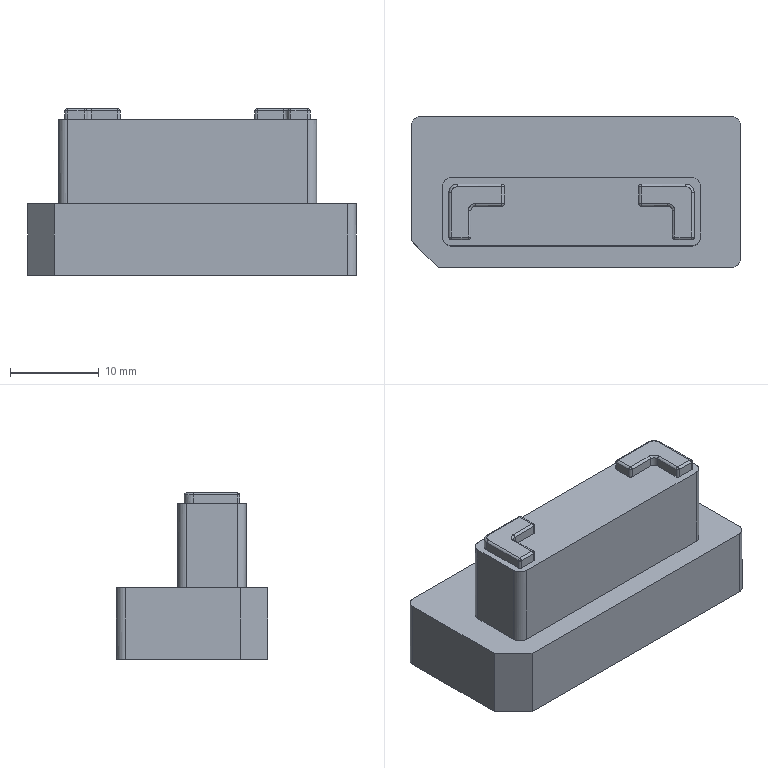NC program | PowerMill | posted with a generic post | part box 37 x 17 x 18.689 mm
Lines 1 to 1026 of 30982:
%
O0001
N104 ( POWERMILL CB  : 2026004.0)
N105 ( POST VER      : 2026.0.0.5161)
N106 ( OPTION FILE   : FANUC)
N107 ( OUTPUT WORKPLANE : WORLD)
N108 (  )
N109 ( TOOL LIST )
N110 (---------------------------------------)
N111 ( NO. | ID        | DIA.| TIP RAD|LENGTH)
N112 (---------------------------------------)
N113 (    1|D10C_1_1_1 |10.0 |  0.0   |74.16 )
N114 (    2|D4C_1      | 4.0 |  0.0   | 59.0 )
N115 (    3|D10_1_1_1  |10.0 |  0.0   |73.84 )
N116 (   10|D3_1       | 3.0 |  0.0   | 58.0 )
N117 (    8|D1_1_1     | 1.0 |  0.0   |56.48 )
N118 (   13|TEXT_D4_1_1| 4.0 |  0.3   |65.96 )
N119 (---------------------------------------)
N120 (  )
N121 ( NUMBER OF TOOLPATHS: 12.0 )
N122 ( ESTIMATED PROGRAM DURATION: 0 HOURS 5 MIN 14 SEC)
N123 (  )
N124 G00 G21 G80 G40 G17
N125 G90
N126 G54
N127 G53 Z0.0
N128 (---------------)
N129 ( START TOOLPATH : 精公开粗01-扫面平行-D10C )
N130 (---------------)
N131 ( TOOL NO.    :1 )
N132 ( TOOL TYPE   : ENDMILL)
N133 ( TOOL ID     : D10C_1_1_1)
N134 ( TOOL DIA    : 10.0 LENGTH 74.16)
N135 T1
N136 M6
N137 S8000 M03
N138 G00 G90 X0.0 Y0.0
N139 G43 Z10.2 H1
N140
N141 G05 P10000 R4
N142 X26.28 Y11.28
N143 Z1.129
N144 G01 Z-0.071 F6000.0
N145 X21.28 F10000.0
N146 X-21.28
N147 Y5.64
N148 X21.28
N149 Y0.0
N150 X-21.28
N151 Y-5.64
N152 X21.28
N153 Y-11.28
N154 X-21.28
N155 X-26.28
N156 G00 Z10.2
N157 G05 P0
N158 (---------------)
N159 ( END TOOLPATH : 精公开粗01-扫面平行-D10C )
N160 (---------------)
N161 ( START TOOLPATH : 精公开粗01-外形偏置-D10C )
N162 (---------------)
N163 G00 X-0.5005 Y-1.2945 Z9.879
N164 G05 P10000 R4
N165 X-28.071 Y-7.1954
N166 Z0.6887
N167 G01 Z-0.5113 F6000.0
N168 X-27.5435 F10000.0
N169 G03 X-22.796 Y-2.4479 I0.0 J4.7475
N170 G01 Y10.28
N171 G02 X-21.796 Y11.28 I1.0 J0.0
N172 G01 X20.795
N173 G02 X21.795 Y10.28 I0.0 J-1.0
N174 G01 Y-2.4477
N175 X18.5751 Y-2.4546
N176 X18.581 Y-5.1616
N177 X18.5136 Y-5.9351
N178 X18.3397 Y-6.7085
N179 X18.0411 Y-7.4819
N180 X17.675 Y-8.1342
N181 X16.9485 Y-9.0288
N182 X16.1282 Y-9.7035
N183 X15.3547 Y-10.1401
N184 X14.5813 Y-10.4291
N185 X13.9308 Y-10.5756
N186 X13.0345 Y-10.6552
N187 X10.7142 Y-10.6411
N188 X9.9408 Y-10.5315
N189 X9.1673 Y-10.3059
N190 X8.3939 Y-9.9485
N191 X8.148 Y-9.8022
N192 X7.6205 Y-9.4268
N193 X7.1765 Y-9.0288
N194 X6.8471 Y-8.6696
N195 X6.532 Y-8.2553
N196 X6.0835 Y-7.4819
N197 X5.8529 Y-6.8783
N198 G03 X5.5469 Y-6.5834 I-0.4671 J-0.1784
N199 G01 X5.3002 Y-6.4994
N200 X4.5268 Y-6.1235
N201 X4.2286 Y-5.9351
N202 X3.7533 Y-5.5756
N203 X3.3753 Y-5.2212
N204 X0.2976 Y-8.5042
N205 X3.3753 Y-5.2212
N206 X3.3117 Y-5.1616
N207 X2.9799 Y-4.7772
N208 X2.6963 Y-4.3882
N209 X2.2692 Y-3.6148
N210 X1.9882 Y-2.8414
N211 X1.8277 Y-2.0679
N212 X1.7748 Y-1.2945
N213 X1.7922 Y1.0258
N214 X1.9084 Y1.7992
N215 X2.1411 Y2.5726
N216 X2.5069 Y3.3461
N217 X2.9799 Y4.0454
N218 X3.7533 Y4.842
N219 X4.5268 Y5.3881
N220 X5.3002 Y5.7645
N221 X6.0736 Y6.0049
N222 X6.8471 Y6.1295
N223 X7.6205 Y6.1515
N224 X12.261
N225 X13.0345 Y6.106
N226 X13.8079 Y5.9707
N227 X14.5813 Y5.7266
N228 X15.3547 Y5.3624
N229 X16.0797 Y4.8929
N230 X16.9016 Y4.153
N231 X17.5329 Y3.3461
N232 X17.9753 Y2.5726
N233 X18.2814 Y1.7992
N234 X18.4484 Y1.168
N235 X18.5693 Y0.2524
N236 X18.5751 Y-2.4546
N237 X21.795 Y-2.4477
N238 Y-12.869
N239 G02 X20.795 Y-13.869 I-1.0 J0.0
N240 G01 X-21.796
N241 G02 X-22.796 Y-12.869 I0.0 J1.0
N242 G01 Y-2.4479
N243 X-19.5753 Y-2.4546
N244 X-19.5696 Y0.2524
N245 X-19.4764 Y1.0258
N246 X-19.2815 Y1.7992
N247 X-18.9753 Y2.5726
N248 X-18.5329 Y3.3461
N249 X-17.9321 Y4.1195
N250 X-17.1292 Y4.8559
N251 X-16.3557 Y5.3618
N252 X-15.7316 Y5.6663
N253 X-14.8089 Y5.9704
N254 X-14.0355 Y6.106
N255 X-13.262 Y6.1515
N256 X-8.6215 Y6.1514
N257 X-7.8481 Y6.1286
N258 X-7.0746 Y6.0018
N259 X-6.3012 Y5.7648
N260 X-5.5278 Y5.3891
N261 X-4.8168 Y4.8929
N262 X-4.0416 Y4.1195
N263 X-3.5069 Y3.3461
N264 X-3.2075 Y2.7386
N265 X-2.913 Y1.7992
N266 X-2.793 Y1.0258
N267 X-2.7748 Y-1.2945
N268 X-2.8251 Y-2.0679
N269 X-2.9864 Y-2.8414
N270 X-3.2075 Y-3.4736
N271 X-3.6959 Y-4.3882
N272 X-3.9809 Y-4.7817
N273 X-4.3117 Y-5.1616
N274 X-4.7543 Y-5.5779
N275 X-5.2295 Y-5.9351
N276 X-5.5278 Y-6.1237
N277 X-6.3012 Y-6.4999
N278 X-6.5485 Y-6.5846
N279 G03 X-6.854 Y-6.8804 I0.1621 J-0.473
N280 G01 X-7.0746 Y-7.4626
N281 X-7.5321 Y-8.2553
N282 X-7.8481 Y-8.6691
N283 X-8.1765 Y-9.0288
N284 X-8.6215 Y-9.4255
N285 X-9.1475 Y-9.8022
N286 X-9.3949 Y-9.9491
N287 X-10.1683 Y-10.3061
N288 X-10.9418 Y-10.5266
N289 X-11.1942 Y-10.5756
N290 X-11.7152 Y-10.6406
N291 X-14.0355 Y-10.6552
N292 X-14.8089 Y-10.5985
N293 X-15.5823 Y-10.4303
N294 X-16.3557 Y-10.1398
N295 X-17.1292 Y-9.7036
N296 X-17.9026 Y-9.074
N297 X-18.593 Y-8.2553
N298 X-19.0416 Y-7.4819
N299 X-19.3412 Y-6.7085
N300 X-19.5171 Y-5.9351
N301 X-19.581 Y-5.1616
N302 X-19.5753 Y-2.4546
N303 X-22.796 Y-2.4479
N304 G00 Z3.2984
N305 G01 X-28.071 Y-7.1954
N306 G00 Z0.2984
N307 G01 Z-0.9016 F6000.0
N308 X-27.5435 F10000.0
N309 G03 X-22.796 Y-2.4479 I0.0 J4.7475
N310 G01 Y10.28
N311 G02 X-21.796 Y11.28 I1.0 J0.0
N312 G01 X20.795
N313 G02 X21.795 Y10.28 I0.0 J-1.0
N314 G01 Y-2.4477
N315 X18.5752 Y-2.4546
N316 X18.581 Y-5.1616
N317 X18.5137 Y-5.9351
N318 X18.3398 Y-6.7085
N319 X18.0412 Y-7.4819
N320 X17.675 Y-8.1342
N321 X16.9486 Y-9.0288
N322 X16.1282 Y-9.7035
N323 X15.3547 Y-10.1402
N324 X14.5813 Y-10.4291
N325 X13.9308 Y-10.5756
N326 X13.0345 Y-10.6552
N327 X10.7142 Y-10.6411
N328 X9.9408 Y-10.5316
N329 X9.1673 Y-10.3059
N330 X8.3939 Y-9.9485
N331 X8.148 Y-9.8022
N332 X7.6205 Y-9.4269
N333 X7.1765 Y-9.0288
N334 X6.8471 Y-8.6696
N335 X6.532 Y-8.2553
N336 X6.0834 Y-7.4819
N337 X5.8529 Y-6.8784
N338 G03 X5.5469 Y-6.5834 I-0.4671 J-0.1783
N339 G01 X5.3002 Y-6.4994
N340 X4.5268 Y-6.1235
N341 X4.2286 Y-5.9351
N342 X3.7533 Y-5.5757
N343 X3.3752 Y-5.2212
N344 X0.2976 Y-8.5042
N345 X3.3752 Y-5.2212
N346 X3.3117 Y-5.1616
N347 X2.9799 Y-4.7773
N348 X2.6963 Y-4.3882
N349 X2.2692 Y-3.6148
N350 X1.9882 Y-2.8414
N351 X1.8277 Y-2.0679
N352 X1.7747 Y-1.2945
N353 X1.7922 Y1.0258
N354 X1.9083 Y1.7992
N355 X2.141 Y2.5726
N356 X2.5069 Y3.3461
N357 X2.9799 Y4.0455
N358 X3.7533 Y4.842
N359 X4.5268 Y5.3881
N360 X5.3002 Y5.7645
N361 X6.0736 Y6.005
N362 X6.8471 Y6.1295
N363 X7.6205 Y6.1515
N364 X12.261
N365 X13.0345 Y6.106
N366 X13.8079 Y5.9707
N367 X14.5813 Y5.7267
N368 X15.3547 Y5.3625
N369 X16.0798 Y4.8929
N370 X16.9016 Y4.1531
N371 X17.533 Y3.3461
N372 X17.9753 Y2.5726
N373 X18.2815 Y1.7992
N374 X18.4484 Y1.168
N375 X18.5693 Y0.2524
N376 X18.5752 Y-2.4546
N377 X21.795 Y-2.4477
N378 Y-12.869
N379 G02 X20.795 Y-13.869 I-1.0 J0.0
N380 G01 X-21.796
N381 G02 X-22.796 Y-12.869 I0.0 J1.0
N382 G01 Y-2.4479
N383 X-19.5754 Y-2.4546
N384 X-19.5697 Y0.2524
N385 X-19.4765 Y1.0258
N386 X-19.2815 Y1.7992
N387 X-18.9753 Y2.5726
N388 X-18.5331 Y3.3461
N389 X-17.9322 Y4.1195
N390 X-17.1292 Y4.8559
N391 X-16.3557 Y5.362
N392 X-15.7316 Y5.6663
N393 X-14.8089 Y5.9705
N394 X-14.0355 Y6.106
N395 X-13.262 Y6.1515
N396 X-8.6215
N397 X-7.8481 Y6.1286
N398 X-7.0746 Y6.0019
N399 X-6.3012 Y5.7649
N400 X-5.5278 Y5.3891
N401 X-4.8168 Y4.8929
N402 X-4.0415 Y4.1195
N403 X-3.5068 Y3.3461
N404 X-3.2075 Y2.7387
N405 X-2.9129 Y1.7992
N406 X-2.793 Y1.0258
N407 X-2.7747 Y-1.2945
N408 X-2.825 Y-2.0679
N409 X-2.9863 Y-2.8414
N410 X-3.2075 Y-3.4737
N411 X-3.6959 Y-4.3882
N412 X-3.9809 Y-4.7817
N413 X-4.3116 Y-5.1616
N414 X-4.7543 Y-5.5779
N415 X-5.2295 Y-5.9351
N416 X-5.5278 Y-6.1237
N417 X-6.3012 Y-6.5
N418 X-6.5484 Y-6.5846
N419 G03 X-6.854 Y-6.8805 I0.162 J-0.4731
N420 G01 X-7.0746 Y-7.4627
N421 X-7.532 Y-8.2553
N422 X-7.8481 Y-8.6692
N423 X-8.1764 Y-9.0288
N424 X-8.6215 Y-9.4255
N425 X-9.1474 Y-9.8022
N426 X-9.3949 Y-9.9491
N427 X-10.1683 Y-10.3061
N428 X-10.9418 Y-10.5266
N429 X-11.1942 Y-10.5756
N430 X-11.7152 Y-10.6406
N431 X-14.0355 Y-10.6552
N432 X-14.8089 Y-10.5986
N433 X-15.5823 Y-10.4303
N434 X-16.3557 Y-10.1399
N435 X-17.1292 Y-9.7036
N436 X-17.9026 Y-9.0741
N437 X-18.593 Y-8.2553
N438 X-19.0417 Y-7.4819
N439 X-19.3412 Y-6.7085
N440 X-19.5171 Y-5.9351
N441 X-19.581 Y-5.1616
N442 X-19.5754 Y-2.4546
N443 X-22.796 Y-2.4479
N444 G00 Z2.9081
N445 G01 X-28.071 Y-7.1954
N446 G00 Z-0.0919
N447 G01 Z-1.2919 F6000.0
N448 X-27.5435 F10000.0
N449 G03 X-22.796 Y-2.4479 I0.0 J4.7475
N450 G01 Y10.28
N451 G02 X-21.796 Y11.28 I1.0 J0.0
N452 G01 X20.795
N453 G02 X21.795 Y10.28 I0.0 J-1.0
N454 G01 Y-2.4477
N455 X18.5752 Y-2.4546
N456 X18.581 Y-5.1616
N457 X18.5137 Y-5.9351
N458 X18.3398 Y-6.7085
N459 X18.0412 Y-7.4819
N460 X17.675 Y-8.1343
N461 X16.9486 Y-9.0288
N462 X16.1282 Y-9.7036
N463 X15.3547 Y-10.1402
N464 X14.5813 Y-10.4292
N465 X13.9309 Y-10.5756
N466 X13.0345 Y-10.6552
N467 X10.7142 Y-10.6411
N468 X9.9408 Y-10.5316
N469 X9.1673 Y-10.306
N470 X8.3939 Y-9.9486
N471 X8.148 Y-9.8022
N472 X7.6205 Y-9.4269
N473 X7.1764 Y-9.0288
N474 X6.8471 Y-8.6697
N475 X6.5319 Y-8.2553
N476 X6.0833 Y-7.4819
N477 X5.8529 Y-6.8784
N478 G03 X5.5468 Y-6.5834 I-0.4671 J-0.1783
N479 G01 X5.3002 Y-6.4995
N480 X4.5268 Y-6.1236
N481 X4.2285 Y-5.9351
N482 X3.7533 Y-5.5757
N483 X3.3752 Y-5.2212
N484 X0.2975 Y-8.5042
N485 X3.3752 Y-5.2212
N486 X3.3116 Y-5.1616
N487 X2.9799 Y-4.7773
N488 X2.6962 Y-4.3882
N489 X2.2691 Y-3.6148
N490 X1.9881 Y-2.8414
N491 X1.8277 Y-2.0679
N492 X1.7747 Y-1.2945
N493 X1.7922 Y1.0258
N494 X1.9083 Y1.7992
N495 X2.141 Y2.5726
N496 X2.5068 Y3.3461
N497 X2.9799 Y4.0455
N498 X3.7533 Y4.8421
N499 X4.5268 Y5.3881
N500 X5.3002 Y5.7646
N501 X6.0736 Y6.005
N502 X6.8471 Y6.1295
N503 X7.6205 Y6.1516
N504 X12.261
N505 X13.0345 Y6.1061
N506 X13.8079 Y5.9707
N507 X14.5813 Y5.7267
N508 X15.3547 Y5.3625
N509 X16.0798 Y4.8929
N510 X16.9016 Y4.1531
N511 X17.533 Y3.3461
N512 X17.9753 Y2.5726
N513 X18.2815 Y1.7992
N514 X18.4484 Y1.168
N515 X18.5693 Y0.2524
N516 X18.5752 Y-2.4546
N517 X21.795 Y-2.4477
N518 Y-12.869
N519 G02 X20.795 Y-13.869 I-1.0 J0.0
N520 G01 X-21.796
N521 G02 X-22.796 Y-12.869 I0.0 J1.0
N522 G01 Y-2.4479
N523 X-19.5754 Y-2.4546
N524 X-19.5697 Y0.2524
N525 X-19.4765 Y1.0258
N526 X-19.2815 Y1.7992
N527 X-18.9753 Y2.5726
N528 X-18.5373 Y3.3461
N529 X-17.9322 Y4.1195
N530 X-17.1292 Y4.8559
N531 X-16.3557 Y5.3622
N532 X-15.7317 Y5.6663
N533 X-14.8089 Y5.9705
N534 X-14.0355 Y6.106
N535 X-13.262 Y6.1516
N536 X-8.6215 Y6.1515
N537 X-7.8481 Y6.1286
N538 X-7.0746 Y6.0019
N539 X-6.3012 Y5.7649
N540 X-5.5278 Y5.3892
N541 X-4.8168 Y4.8929
N542 X-4.0415 Y4.1195
N543 X-3.5068 Y3.3461
N544 X-3.2075 Y2.7388
N545 X-2.9129 Y1.7992
N546 X-2.793 Y1.0258
N547 X-2.7747 Y-1.2945
N548 X-2.825 Y-2.0679
N549 X-2.9863 Y-2.8414
N550 X-3.2075 Y-3.4737
N551 X-3.6958 Y-4.3882
N552 X-3.9809 Y-4.7818
N553 X-4.3116 Y-5.1616
N554 X-4.7543 Y-5.5779
N555 X-5.2294 Y-5.9351
N556 X-5.5278 Y-6.1237
N557 X-6.3012 Y-6.5
N558 X-6.5488 Y-6.5848
N559 X-6.5752 Y-6.5946
N560 X-6.6009 Y-6.6059
N561 G03 X-6.854 Y-6.8804 I0.2145 J-0.4518
N562 G01 X-7.0369 Y-7.3629
N563 X-7.0746 Y-7.4627
N564 X-7.532 Y-8.2553
N565 X-7.8481 Y-8.6692
N566 X-8.1764 Y-9.0288
N567 X-8.6215 Y-9.4255
N568 X-9.1474 Y-9.8022
N569 X-9.3949 Y-9.9491
N570 X-10.1683 Y-10.3062
N571 X-10.9418 Y-10.5267
N572 X-11.1941 Y-10.5756
N573 X-11.7152 Y-10.6406
N574 X-14.0355 Y-10.6552
N575 X-14.8089 Y-10.5986
N576 X-15.5823 Y-10.4304
N577 X-16.3557 Y-10.1399
N578 X-17.1292 Y-9.7037
N579 X-17.9026 Y-9.0741
N580 X-18.5931 Y-8.2553
N581 X-19.0417 Y-7.4819
N582 X-19.3412 Y-6.7085
N583 X-19.5172 Y-5.9351
N584 X-19.5811 Y-5.1616
N585 X-19.5754 Y-2.4546
N586 X-22.796 Y-2.4479
N587 G00 Z2.5161
N588 G01 X-28.071 Y-7.1954
N589 G00 Z-0.4839
N590 G01 Z-1.6839 F6000.0
N591 X-27.5435 F10000.0
N592 G03 X-22.796 Y-2.4479 I0.0 J4.7475
N593 G01 Y10.28
N594 G02 X-21.796 Y11.28 I1.0 J0.0
N595 G01 X20.795
N596 G02 X21.795 Y10.28 I0.0 J-1.0
N597 G01 Y1.0853
N598 X19.2789 Y1.0258
N599 X19.2972 Y0.2524
N600 X19.2968 Y-5.1616
N601 X19.233 Y-5.9351
N602 X19.0852 Y-6.7085
N603 X18.8205 Y-7.4819
N604 X18.4484 Y-8.2436
N605 X17.9074 Y-9.0288
N606 X17.675 Y-9.301
N607 X17.166 Y-9.8022
N608 X16.9016 Y-10.0244
N609 X16.1282 Y-10.5462
N610 X15.3547 Y-10.9168
N611 X14.5813 Y-11.173
N612 X13.4982 Y-11.349
N613 X13.0345 Y-11.3709
N614 X-14.0355
N615 X-14.4982 Y-11.349
N616 X-15.5823 Y-11.1728
N617 X-16.3557 Y-10.9164
N618 X-17.0762 Y-10.5756
N619 X-17.9026 Y-10.0236
N620 X-18.1661 Y-9.8022
N621 X-18.676 Y-9.2999
N622 X-18.9074 Y-9.0288
N623 X-19.4415 Y-8.2553
N624 X-19.8205 Y-7.4819
N625 X-20.0853 Y-6.7085
N626 X-20.2229 Y-6.0163
N627 X-20.2968 Y-5.1616
N628 X-20.2972 Y0.2524
N629 X-20.279 Y1.0258
N630 X-20.1775 Y1.7992
N631 X-19.9751 Y2.5726
N632 X-19.6567 Y3.3461
N633 X-19.4494 Y3.7381
N634 X-19.209 Y4.1195
N635 X-18.676 Y4.7962
N636 X-17.9026 Y5.5199
N637 X-17.1292 Y6.0419
N638 X-16.3557 Y6.4126
N639 X-15.5823 Y6.6691
N640 X-14.8089 Y6.8095
N641 X-14.0355 Y6.8672
N642 X13.0345
N643 X13.8079 Y6.8096
N644 X14.5813 Y6.6693
N645 X15.2894 Y6.4398
N646 X16.1282 Y6.0425
N647 X16.9016 Y5.5207
N648 X17.5881 Y4.8929
N649 X18.209 Y4.1195
N650 X18.4484 Y3.7398
N651 X18.6567 Y3.3461
N652 X18.9751 Y2.5726
N653 X19.1775 Y1.7992
N654 X19.2789 Y1.0258
N655 X21.795 Y1.0853
N656 Y-12.869
N657 G02 X20.795 Y-13.869 I-1.0 J0.0
N658 G01 X-21.796
N659 G02 X-22.796 Y-12.869 I0.0 J1.0
N660 G01 Y-2.4479
N661 G00 Z2.1241
N662 G01 X-28.071 Y-7.1954
N663 G00 Z-0.8759
N664 G01 Z-2.0759 F6000.0
N665 X-27.5435 F10000.0
N666 G03 X-22.796 Y-2.4479 I0.0 J4.7475
N667 G01 Y10.28
N668 G02 X-21.796 Y11.28 I1.0 J0.0
N669 G01 X20.795
N670 G02 X21.795 Y10.28 I0.0 J-1.0
N671 G01 Y1.0853
N672 X19.2789 Y1.0258
N673 X19.2972 Y0.2524
N674 X19.2968 Y-5.1616
N675 X19.233 Y-5.9351
N676 X19.0852 Y-6.7085
N677 X18.8205 Y-7.4819
N678 X18.4484 Y-8.2436
N679 X17.9074 Y-9.0288
N680 X17.675 Y-9.301
N681 X17.166 Y-9.8022
N682 X16.9016 Y-10.0244
N683 X16.1282 Y-10.5462
N684 X15.3547 Y-10.9168
N685 X14.5813 Y-11.173
N686 X13.4982 Y-11.349
N687 X13.0345 Y-11.3709
N688 X-14.0355
N689 X-14.4982 Y-11.349
N690 X-15.5823 Y-11.1728
N691 X-16.3557 Y-10.9164
N692 X-17.0762 Y-10.5756
N693 X-17.9026 Y-10.0236
N694 X-18.1661 Y-9.8022
N695 X-18.676 Y-9.2999
N696 X-18.9074 Y-9.0288
N697 X-19.4415 Y-8.2553
N698 X-19.8205 Y-7.4819
N699 X-20.0853 Y-6.7085
N700 X-20.2229 Y-6.0163
N701 X-20.2968 Y-5.1616
N702 X-20.2972 Y0.2524
N703 X-20.279 Y1.0258
N704 X-20.1775 Y1.7992
N705 X-19.9751 Y2.5726
N706 X-19.6567 Y3.3461
N707 X-19.4494 Y3.7381
N708 X-19.209 Y4.1195
N709 X-18.676 Y4.7962
N710 X-17.9026 Y5.5199
N711 X-17.1292 Y6.0419
N712 X-16.3557 Y6.4126
N713 X-15.5823 Y6.6691
N714 X-14.8089 Y6.8095
N715 X-14.0355 Y6.8672
N716 X13.0345
N717 X13.8079 Y6.8096
N718 X14.5813 Y6.6693
N719 X15.2894 Y6.4398
N720 X16.1282 Y6.0425
N721 X16.9016 Y5.5207
N722 X17.5881 Y4.8929
N723 X18.209 Y4.1195
N724 X18.4484 Y3.7398
N725 X18.6567 Y3.3461
N726 X18.9751 Y2.5726
N727 X19.1775 Y1.7992
N728 X19.2789 Y1.0258
N729 X21.795 Y1.0853
N730 Y-12.869
N731 G02 X20.795 Y-13.869 I-1.0 J0.0
N732 G01 X-21.796
N733 G02 X-22.796 Y-12.869 I0.0 J1.0
N734 G01 Y-2.4479
N735 G00 Z1.7321
N736 G01 X-28.071 Y-7.1954
N737 G00 Z-1.2679
N738 G01 Z-2.4679 F6000.0
N739 X-27.5435 F10000.0
N740 G03 X-22.796 Y-2.4479 I0.0 J4.7475
N741 G01 Y10.28
N742 G02 X-21.796 Y11.28 I1.0 J0.0
N743 G01 X20.795
N744 G02 X21.795 Y10.28 I0.0 J-1.0
N745 G01 Y1.0853
N746 X19.2789 Y1.0258
N747 X19.2972 Y0.2524
N748 X19.2968 Y-5.1616
N749 X19.233 Y-5.9351
N750 X19.0852 Y-6.7085
N751 X18.8205 Y-7.4819
N752 X18.4484 Y-8.2436
N753 X17.9074 Y-9.0288
N754 X17.675 Y-9.301
N755 X17.166 Y-9.8022
N756 X16.9016 Y-10.0244
N757 X16.1282 Y-10.5462
N758 X15.3547 Y-10.9168
N759 X14.5813 Y-11.173
N760 X13.4982 Y-11.349
N761 X13.0345 Y-11.3709
N762 X-14.0355
N763 X-14.4982 Y-11.349
N764 X-15.5823 Y-11.1728
N765 X-16.3557 Y-10.9164
N766 X-17.0762 Y-10.5756
N767 X-17.9026 Y-10.0236
N768 X-18.1661 Y-9.8022
N769 X-18.676 Y-9.2999
N770 X-18.9074 Y-9.0288
N771 X-19.4415 Y-8.2553
N772 X-19.8205 Y-7.4819
N773 X-20.0853 Y-6.7085
N774 X-20.2229 Y-6.0163
N775 X-20.2968 Y-5.1616
N776 X-20.2972 Y0.2524
N777 X-20.279 Y1.0258
N778 X-20.1775 Y1.7992
N779 X-19.9751 Y2.5726
N780 X-19.6567 Y3.3461
N781 X-19.4494 Y3.7381
N782 X-19.209 Y4.1195
N783 X-18.676 Y4.7962
N784 X-17.9026 Y5.5199
N785 X-17.1292 Y6.0419
N786 X-16.3557 Y6.4126
N787 X-15.5823 Y6.6691
N788 X-14.8089 Y6.8096
N789 X-14.0355 Y6.8672
N790 X13.0345
N791 X13.8079 Y6.8096
N792 X14.5813 Y6.6693
N793 X15.2894 Y6.4398
N794 X16.1282 Y6.0425
N795 X16.9016 Y5.5207
N796 X17.5881 Y4.8929
N797 X18.209 Y4.1195
N798 X18.4484 Y3.7398
N799 X18.6567 Y3.3461
N800 X18.9751 Y2.5726
N801 X19.1775 Y1.7992
N802 X19.2789 Y1.0258
N803 X21.795 Y1.0853
N804 Y-12.869
N805 G02 X20.795 Y-13.869 I-1.0 J0.0
N806 G01 X-21.796
N807 G02 X-22.796 Y-12.869 I0.0 J1.0
N808 G01 Y-2.4479
N809 G00 Z1.3401
N810 G01 X-28.071 Y-7.1954
N811 G00 Z-1.6599
N812 G01 Z-2.8599 F6000.0
N813 X-27.5435 F10000.0
N814 G03 X-22.796 Y-2.4479 I0.0 J4.7475
N815 G01 Y10.28
N816 G02 X-21.796 Y11.28 I1.0 J0.0
N817 G01 X20.795
N818 G02 X21.795 Y10.28 I0.0 J-1.0
N819 G01 Y1.0853
N820 X19.2789 Y1.0258
N821 X19.2972 Y0.2524
N822 X19.2968 Y-5.1616
N823 X19.233 Y-5.9351
N824 X19.0852 Y-6.7085
N825 X18.8205 Y-7.4819
N826 X18.4484 Y-8.2436
N827 X17.9074 Y-9.0288
N828 X17.675 Y-9.301
N829 X17.166 Y-9.8022
N830 X16.9016 Y-10.0244
N831 X16.1282 Y-10.5462
N832 X15.3547 Y-10.9168
N833 X14.5813 Y-11.173
N834 X13.4982 Y-11.349
N835 X13.0345 Y-11.3709
N836 X-14.0355
N837 X-14.4982 Y-11.349
N838 X-15.5823 Y-11.1728
N839 X-16.3557 Y-10.9164
N840 X-17.0762 Y-10.5756
N841 X-17.9026 Y-10.0236
N842 X-18.1661 Y-9.8022
N843 X-18.676 Y-9.2999
N844 X-18.9074 Y-9.0288
N845 X-19.4415 Y-8.2553
N846 X-19.8205 Y-7.4819
N847 X-20.0853 Y-6.7085
N848 X-20.2229 Y-6.0163
N849 X-20.2968 Y-5.1616
N850 X-20.2973 Y0.2524
N851 X-20.279 Y1.0258
N852 X-20.1775 Y1.7992
N853 X-19.9751 Y2.5726
N854 X-19.6567 Y3.3461
N855 X-19.4494 Y3.7381
N856 X-19.209 Y4.1195
N857 X-18.676 Y4.7962
N858 X-17.9026 Y5.5199
N859 X-17.1292 Y6.0419
N860 X-16.3557 Y6.4127
N861 X-15.5823 Y6.6691
N862 X-14.8089 Y6.8096
N863 X-14.0355 Y6.8672
N864 X13.0345
N865 X13.8079 Y6.8096
N866 X14.5813 Y6.6693
N867 X15.2894 Y6.4398
N868 X16.1282 Y6.0425
N869 X16.9016 Y5.5207
N870 X17.5881 Y4.8929
N871 X18.209 Y4.1195
N872 X18.4484 Y3.7398
N873 X18.6567 Y3.3461
N874 X18.9751 Y2.5726
N875 X19.1775 Y1.7992
N876 X19.2789 Y1.0258
N877 X21.795 Y1.0853
N878 Y-12.869
N879 G02 X20.795 Y-13.869 I-1.0 J0.0
N880 G01 X-21.796
N881 G02 X-22.796 Y-12.869 I0.0 J1.0
N882 G01 Y-2.4479
N883 G00 Z0.9481
N884 G01 X-28.071 Y-7.1954
N885 G00 Z-2.0519
N886 G01 Z-3.2519 F6000.0
N887 X-27.5435 F10000.0
N888 G03 X-22.796 Y-2.4479 I0.0 J4.7475
N889 G01 Y10.28
N890 G02 X-21.796 Y11.28 I1.0 J0.0
N891 G01 X20.795
N892 G02 X21.795 Y10.28 I0.0 J-1.0
N893 G01 Y1.0853
N894 X19.2789 Y1.0258
N895 X19.2972 Y0.2524
N896 X19.2968 Y-5.1616
N897 X19.233 Y-5.9351
N898 X19.0852 Y-6.7085
N899 X18.8205 Y-7.4819
N900 X18.4484 Y-8.2436
N901 X17.9074 Y-9.0288
N902 X17.675 Y-9.301
N903 X17.166 Y-9.8022
N904 X16.9016 Y-10.0244
N905 X16.1282 Y-10.5462
N906 X15.3547 Y-10.9168
N907 X14.5813 Y-11.1731
N908 X13.4982 Y-11.349
N909 X13.0345 Y-11.3709
N910 X-14.0355
N911 X-14.4982 Y-11.349
N912 X-15.5823 Y-11.1728
N913 X-16.3557 Y-10.9164
N914 X-17.0762 Y-10.5756
N915 X-17.9026 Y-10.0236
N916 X-18.1661 Y-9.8022
N917 X-18.676 Y-9.2999
N918 X-18.9074 Y-9.0288
N919 X-19.4415 Y-8.2553
N920 X-19.8205 Y-7.4819
N921 X-20.0853 Y-6.7085
N922 X-20.2229 Y-6.0163
N923 X-20.2968 Y-5.1616
N924 X-20.2973 Y0.2524
N925 X-20.279 Y1.0258
N926 X-20.1775 Y1.7992
N927 X-19.9751 Y2.5726
N928 X-19.6567 Y3.3461
N929 X-19.4494 Y3.7381
N930 X-19.209 Y4.1195
N931 X-18.676 Y4.7962
N932 X-17.9026 Y5.5199
N933 X-17.1292 Y6.0419
N934 X-16.3557 Y6.4127
N935 X-15.5823 Y6.6691
N936 X-14.8089 Y6.8096
N937 X-14.0355 Y6.8672
N938 X13.0345
N939 X13.8079 Y6.8096
N940 X14.5813 Y6.6694
N941 X15.2894 Y6.4398
N942 X16.1282 Y6.0425
N943 X16.9016 Y5.5207
N944 X17.5881 Y4.8929
N945 X18.209 Y4.1195
N946 X18.4484 Y3.7398
N947 X18.6567 Y3.3461
N948 X18.9751 Y2.5726
N949 X19.1775 Y1.7992
N950 X19.2789 Y1.0258
N951 X21.795 Y1.0853
N952 Y-12.869
N953 G02 X20.795 Y-13.869 I-1.0 J0.0
N954 G01 X-21.796
N955 G02 X-22.796 Y-12.869 I0.0 J1.0
N956 G01 Y-2.4479
N957 G00 Z0.5561
N958 G01 X-28.071 Y-7.1954
N959 G00 Z-2.4439
N960 G01 Z-3.6439 F6000.0
N961 X-27.5435 F10000.0
N962 G03 X-22.796 Y-2.4479 I0.0 J4.7475
N963 G01 Y10.28
N964 G02 X-21.796 Y11.28 I1.0 J0.0
N965 G01 X20.795
N966 G02 X21.795 Y10.28 I0.0 J-1.0
N967 G01 Y1.0853
N968 X19.2789 Y1.0258
N969 X19.2972 Y0.2524
N970 X19.2968 Y-5.1616
N971 X19.233 Y-5.9351
N972 X19.0852 Y-6.7085
N973 X18.8205 Y-7.4819
N974 X18.4484 Y-8.2436
N975 X17.9074 Y-9.0288
N976 X17.675 Y-9.301
N977 X17.166 Y-9.8022
N978 X16.9016 Y-10.0245
N979 X16.1282 Y-10.5462
N980 X15.3547 Y-10.9168
N981 X14.5813 Y-11.1731
N982 X13.4982 Y-11.349
N983 X13.0345 Y-11.3709
N984 X-14.0355
N985 X-14.4982 Y-11.349
N986 X-15.5823 Y-11.1728
N987 X-16.3557 Y-10.9164
N988 X-17.0762 Y-10.5756
N989 X-17.9026 Y-10.0236
N990 X-18.1661 Y-9.8022
N991 X-18.676 Y-9.2999
N992 X-18.9074 Y-9.0288
N993 X-19.4415 Y-8.2553
N994 X-19.8206 Y-7.4819
N995 X-20.0853 Y-6.7085
N996 X-20.2229 Y-6.0163
N997 X-20.2968 Y-5.1616
N998 X-20.2973 Y0.2524
N999 X-20.279 Y1.0258
N1000 X-20.1775 Y1.7992
N1001 X-19.9751 Y2.5726
N1002 X-19.6567 Y3.3461
N1003 X-19.4494 Y3.7381
N1004 X-19.209 Y4.1195
N1005 X-18.676 Y4.7962
N1006 X-17.9026 Y5.5199
N1007 X-17.1292 Y6.0419
N1008 X-16.3557 Y6.4127
N1009 X-15.5823 Y6.6691
N1010 X-14.8089 Y6.8096
N1011 X-14.0355 Y6.8672
N1012 X13.0345
N1013 X13.8079 Y6.8096
N1014 X14.5813 Y6.6694
N1015 X15.2894 Y6.4398
N1016 X16.1282 Y6.0425
N1017 X16.9016 Y5.5207
N1018 X17.5881 Y4.8929
N1019 X18.209 Y4.1195
N1020 X18.4484 Y3.7399
N1021 X18.6567 Y3.3461
N1022 X18.9751 Y2.5726
N1023 X19.1775 Y1.7992
N1024 X19.2789 Y1.0258
N1025 X21.795 Y1.0853
N1026 Y-12.869
N1027 G02 X20.795 Y-13.869 I-1.0 J0.0
N1028 G01 X-21.796
N1029 G02 X-22.796 Y-12.869 I0.0 J1.0
N1030 G01 Y-2.4479
N1031 G00 Z0.1641
N1032 G01 X-28.071 Y-7.1954
N1033 G00 Z-2.8359
N1034 G01 Z-4.0359 F6000.0
N1035 X-27.5435 F10000.0
N1036 G03 X-22.796 Y-2.4479 I0.0 J4.7475
N1037 G01 Y10.28
N1038 G02 X-21.796 Y11.28 I1.0 J0.0
N1039 G01 X20.795
N1040 G02 X21.795 Y10.28 I0.0 J-1.0
N1041 G01 Y1.0853
N1042 X19.2789 Y1.0258
N1043 X19.2972 Y0.2524
N1044 X19.2968 Y-5.1616
N1045 X19.233 Y-5.9351
N1046 X19.0852 Y-6.7085
N1047 X18.8205 Y-7.4819
N1048 X18.4484 Y-8.2436
N1049 X17.9074 Y-9.0288
N1050 X17.675 Y-9.3011
N1051 X17.1661 Y-9.8022
N1052 X16.9016 Y-10.0245
N1053 X16.1282 Y-10.5462
N1054 X15.3547 Y-10.9168
N1055 X14.5813 Y-11.1731
N1056 X13.4982 Y-11.349
N1057 X13.0345 Y-11.3709
N1058 X-14.0355
N1059 X-14.4982 Y-11.349
N1060 X-15.5823 Y-11.1728
N1061 X-16.3557 Y-10.9164
N1062 X-17.0762 Y-10.5756
N1063 X-17.9026 Y-10.0236
N1064 X-18.1661 Y-9.8022
N1065 X-18.676 Y-9.2999
N1066 X-18.9074 Y-9.0288
N1067 X-19.4415 Y-8.2553
N1068 X-19.8206 Y-7.4819
N1069 X-20.0853 Y-6.7085
N1070 X-20.2229 Y-6.0163
N1071 X-20.2968 Y-5.1616
N1072 X-20.2973 Y0.2524
N1073 X-20.279 Y1.0258
N1074 X-20.1775 Y1.7992
N1075 X-19.9751 Y2.5726
N1076 X-19.6567 Y3.3461
N1077 X-19.4494 Y3.7381
N1078 X-19.209 Y4.1195
N1079 X-18.676 Y4.7962
N1080 X-17.9026 Y5.5199
N1081 X-17.1292 Y6.0419
N1082 X-16.3557 Y6.4127
N1083 X-15.5823 Y6.6691
N1084 X-14.8089 Y6.8096
N1085 X-14.0355 Y6.8672
N1086 X13.0345
N1087 X13.8079 Y6.8096
N1088 X14.5813 Y6.6694
N1089 X15.2894 Y6.4398
N1090 X16.1282 Y6.0425
N1091 X16.9016 Y5.5207
N1092 X17.5881 Y4.8929
N1093 X18.209 Y4.1195
N1094 X18.4484 Y3.7399
N1095 X18.6567 Y3.3461
N1096 X18.9751 Y2.5726
N1097 X19.1775 Y1.7992
N1098 X19.2789 Y1.0258
N1099 X21.795 Y1.0853
N1100 Y-12.869
N1101 G02 X20.795 Y-13.869 I-1.0 J0.0
N1102 G01 X-21.796
N1103 G02 X-22.796 Y-12.869 I0.0 J1.0
N1104 G01 Y-2.4479
N1105 G00 Z-0.2279
N1106 G01 X-28.071 Y-7.1954
N1107 G00 Z-3.2279
N1108 G01 Z-4.4279 F6000.0
N1109 X-27.5435 F10000.0
N1110 G03 X-22.796 Y-2.4479 I0.0 J4.7475
N1111 G01 Y10.28
N1112 G02 X-21.796 Y11.28 I1.0 J0.0
N1113 G01 X20.795
N1114 G02 X21.795 Y10.28 I0.0 J-1.0
N1115 G01 Y1.0853
N1116 X19.279 Y1.0258
N1117 X19.2972 Y0.2524
N1118 X19.2968 Y-5.1616
N1119 X19.233 Y-5.9351
N1120 X19.0852 Y-6.7085
N1121 X18.8205 Y-7.4819
N1122 X18.4484 Y-8.2436
N1123 X17.9074 Y-9.0288